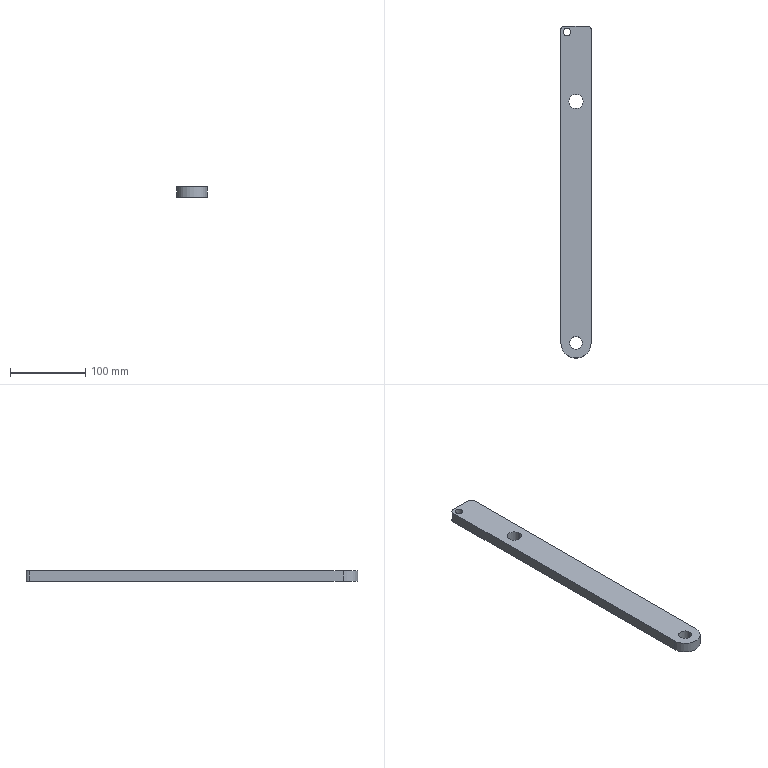Part | SolidWorks | features Extrusion 1, ICE 1 | 1 solid | 14 faces | box 40 x 440 x 14 mm | volume 235600 mm3 | cylinder 9 | plane 5 | commonest cylinder face diameters 10 x4 17 x2 19 x2 40 x1
STEP:
#1=CARTESIAN_POINT('',(-7.,212.,14.));
#2=VERTEX_POINT('',#1);
#3=CARTESIAN_POINT('',(-17.,212.,14.));
#4=VERTEX_POINT('',#3);
#5=CARTESIAN_POINT('',(-12.,212.,14.));
#6=DIRECTION('',(0.,0.,-1.));
#7=DIRECTION('',(-1.,0.,0.));
#8=AXIS2_PLACEMENT_3D('',#5,#6,#7);
#9=CIRCLE('',#8,5.);
#10=EDGE_CURVE('',#2,#4,#9,.T.);
#11=ORIENTED_EDGE('',*,*,#10,.F.);
#12=CARTESIAN_POINT('',(-7.,212.,0.));
#13=VERTEX_POINT('',#12);
#14=CARTESIAN_POINT('',(-7.,212.,20.));
#15=DIRECTION('',(0.,0.,-1.));
#16=VECTOR('',#15,1000.);
#17=LINE('',#14,#16);
#18=EDGE_CURVE('',#2,#13,#17,.T.);
#19=ORIENTED_EDGE('',*,*,#18,.T.);
#20=CARTESIAN_POINT('',(-17.,212.,0.));
#21=VERTEX_POINT('',#20);
#22=CARTESIAN_POINT('',(-12.,212.,0.));
#23=DIRECTION('',(0.,0.,-1.));
#24=DIRECTION('',(-1.,0.,0.));
#25=AXIS2_PLACEMENT_3D('',#22,#23,#24);
#26=CIRCLE('',#25,5.);
#27=EDGE_CURVE('',#13,#21,#26,.T.);
#28=ORIENTED_EDGE('',*,*,#27,.T.);
#29=CARTESIAN_POINT('',(-17.,212.,20.));
#30=DIRECTION('',(0.,0.,-1.));
#31=VECTOR('',#30,1000.);
#32=LINE('',#29,#31);
#33=EDGE_CURVE('',#4,#21,#32,.T.);
#34=ORIENTED_EDGE('',*,*,#33,.F.);
#35=EDGE_LOOP('',(#11,#19,#28,#34));
#36=FACE_OUTER_BOUND('',#35,.T.);
#37=CARTESIAN_POINT('',(-12.,212.,20.));
#38=DIRECTION('',(0.,0.,-1.));
#39=DIRECTION('',(-1.,0.,0.));
#40=AXIS2_PLACEMENT_3D('',#37,#38,#39);
#41=CYLINDRICAL_SURFACE('',#40,5.);
#42=ADVANCED_FACE('',(#36),#41,.F.);
#43=CARTESIAN_POINT('',(-8.5,-200.,14.));
#44=VERTEX_POINT('',#43);
#45=CARTESIAN_POINT('',(8.5,-200.,14.));
#46=VERTEX_POINT('',#45);
#47=CARTESIAN_POINT('',(0.,-200.,14.));
#48=DIRECTION('',(0.,0.,1.));
#49=DIRECTION('',(1.,0.,0.));
#50=AXIS2_PLACEMENT_3D('',#47,#48,#49);
#51=CIRCLE('',#50,8.5);
#52=EDGE_CURVE('',#44,#46,#51,.T.);
#53=ORIENTED_EDGE('',*,*,#52,.T.);
#54=CARTESIAN_POINT('',(8.5,-200.,0.));
#55=VERTEX_POINT('',#54);
#56=CARTESIAN_POINT('',(8.5,-200.,14.));
#57=DIRECTION('',(0.,0.,-1.));
#58=VECTOR('',#57,1000.);
#59=LINE('',#56,#58);
#60=EDGE_CURVE('',#46,#55,#59,.T.);
#61=ORIENTED_EDGE('',*,*,#60,.T.);
#62=CARTESIAN_POINT('',(-8.5,-200.,0.));
#63=VERTEX_POINT('',#62);
#64=CARTESIAN_POINT('',(0.,-200.,0.));
#65=DIRECTION('',(0.,0.,1.));
#66=DIRECTION('',(1.,0.,0.));
#67=AXIS2_PLACEMENT_3D('',#64,#65,#66);
#68=CIRCLE('',#67,8.5);
#69=EDGE_CURVE('',#63,#55,#68,.T.);
#70=ORIENTED_EDGE('',*,*,#69,.F.);
#71=CARTESIAN_POINT('',(-8.5,-200.,14.));
#72=DIRECTION('',(0.,0.,-1.));
#73=VECTOR('',#72,1000.);
#74=LINE('',#71,#73);
#75=EDGE_CURVE('',#44,#63,#74,.T.);
#76=ORIENTED_EDGE('',*,*,#75,.F.);
#77=EDGE_LOOP('',(#53,#61,#70,#76));
#78=FACE_OUTER_BOUND('',#77,.T.);
#79=CARTESIAN_POINT('',(0.,-200.,14.));
#80=DIRECTION('',(0.,0.,-1.));
#81=DIRECTION('',(-1.,0.,0.));
#82=AXIS2_PLACEMENT_3D('',#79,#80,#81);
#83=CYLINDRICAL_SURFACE('',#82,8.5);
#84=ADVANCED_FACE('',(#78),#83,.F.);
#85=CARTESIAN_POINT('',(-9.5,120.,14.));
#86=VERTEX_POINT('',#85);
#87=CARTESIAN_POINT('',(9.5,120.,14.));
#88=VERTEX_POINT('',#87);
#89=CARTESIAN_POINT('',(0.,120.,14.));
#90=DIRECTION('',(0.,0.,1.));
#91=DIRECTION('',(1.,0.,0.));
#92=AXIS2_PLACEMENT_3D('',#89,#90,#91);
#93=CIRCLE('',#92,9.5);
#94=EDGE_CURVE('',#86,#88,#93,.T.);
#95=ORIENTED_EDGE('',*,*,#94,.T.);
#96=CARTESIAN_POINT('',(9.5,120.,0.));
#97=VERTEX_POINT('',#96);
#98=CARTESIAN_POINT('',(9.5,120.,14.));
#99=DIRECTION('',(0.,0.,-1.));
#100=VECTOR('',#99,1000.);
#101=LINE('',#98,#100);
#102=EDGE_CURVE('',#88,#97,#101,.T.);
#103=ORIENTED_EDGE('',*,*,#102,.T.);
#104=CARTESIAN_POINT('',(-9.5,120.,0.));
#105=VERTEX_POINT('',#104);
#106=CARTESIAN_POINT('',(0.,120.,0.));
#107=DIRECTION('',(0.,0.,1.));
#108=DIRECTION('',(1.,0.,0.));
#109=AXIS2_PLACEMENT_3D('',#106,#107,#108);
#110=CIRCLE('',#109,9.5);
#111=EDGE_CURVE('',#105,#97,#110,.T.);
#112=ORIENTED_EDGE('',*,*,#111,.F.);
#113=CARTESIAN_POINT('',(-9.5,120.,14.));
#114=DIRECTION('',(0.,0.,-1.));
#115=VECTOR('',#114,1000.);
#116=LINE('',#113,#115);
#117=EDGE_CURVE('',#86,#105,#116,.T.);
#118=ORIENTED_EDGE('',*,*,#117,.F.);
#119=EDGE_LOOP('',(#95,#103,#112,#118));
#120=FACE_OUTER_BOUND('',#119,.T.);
#121=CARTESIAN_POINT('',(0.,120.,14.));
#122=DIRECTION('',(0.,0.,-1.));
#123=DIRECTION('',(-1.,0.,0.));
#124=AXIS2_PLACEMENT_3D('',#121,#122,#123);
#125=CYLINDRICAL_SURFACE('',#124,9.5);
#126=ADVANCED_FACE('',(#120),#125,.F.);
#127=CARTESIAN_POINT('',(-12.,212.,14.));
#128=DIRECTION('',(0.,0.,-1.));
#129=DIRECTION('',(-1.,0.,0.));
#130=AXIS2_PLACEMENT_3D('',#127,#128,#129);
#131=CIRCLE('',#130,5.);
#132=EDGE_CURVE('',#4,#2,#131,.T.);
#133=ORIENTED_EDGE('',*,*,#132,.T.);
#134=ORIENTED_EDGE('',*,*,#10,.T.);
#135=EDGE_LOOP('',(#133,#134));
#136=FACE_BOUND('',#135,.T.);
#137=CARTESIAN_POINT('',(20.,215.,14.));
#138=VERTEX_POINT('',#137);
#139=CARTESIAN_POINT('',(15.,220.,14.));
#140=VERTEX_POINT('',#139);
#141=CARTESIAN_POINT('',(15.,215.,14.));
#142=DIRECTION('',(0.,0.,1.));
#143=DIRECTION('',(-1.,0.,0.));
#144=AXIS2_PLACEMENT_3D('',#141,#142,#143);
#145=CIRCLE('',#144,5.);
#146=EDGE_CURVE('',#138,#140,#145,.T.);
#147=ORIENTED_EDGE('',*,*,#146,.T.);
#148=CARTESIAN_POINT('',(-15.,220.,14.));
#149=VERTEX_POINT('',#148);
#150=CARTESIAN_POINT('',(-15.,220.,14.));
#151=DIRECTION('',(-1.,0.,0.));
#152=VECTOR('',#151,1000.);
#153=LINE('',#150,#152);
#154=EDGE_CURVE('',#140,#149,#153,.T.);
#155=ORIENTED_EDGE('',*,*,#154,.T.);
#156=CARTESIAN_POINT('',(-20.,215.,14.));
#157=VERTEX_POINT('',#156);
#158=CARTESIAN_POINT('',(-15.,215.,14.));
#159=DIRECTION('',(0.,0.,1.));
#160=DIRECTION('',(1.,0.,0.));
#161=AXIS2_PLACEMENT_3D('',#158,#159,#160);
#162=CIRCLE('',#161,5.);
#163=EDGE_CURVE('',#149,#157,#162,.T.);
#164=ORIENTED_EDGE('',*,*,#163,.T.);
#165=CARTESIAN_POINT('',(-20.,-200.,14.));
#166=VERTEX_POINT('',#165);
#167=CARTESIAN_POINT('',(-20.,215.,14.));
#168=DIRECTION('',(0.,-1.,0.));
#169=VECTOR('',#168,1000.);
#170=LINE('',#167,#169);
#171=EDGE_CURVE('',#157,#166,#170,.T.);
#172=ORIENTED_EDGE('',*,*,#171,.T.);
#173=CARTESIAN_POINT('',(20.,-200.,14.));
#174=VERTEX_POINT('',#173);
#175=CARTESIAN_POINT('',(0.,-200.,14.));
#176=DIRECTION('',(0.,0.,1.));
#177=DIRECTION('',(1.,0.,0.));
#178=AXIS2_PLACEMENT_3D('',#175,#176,#177);
#179=CIRCLE('',#178,20.);
#180=EDGE_CURVE('',#166,#174,#179,.T.);
#181=ORIENTED_EDGE('',*,*,#180,.T.);
#182=CARTESIAN_POINT('',(20.,215.,14.));
#183=DIRECTION('',(0.,1.,0.));
#184=VECTOR('',#183,1000.);
#185=LINE('',#182,#184);
#186=EDGE_CURVE('',#174,#138,#185,.T.);
#187=ORIENTED_EDGE('',*,*,#186,.T.);
#188=EDGE_LOOP('',(#147,#155,#164,#172,#181,#187));
#189=FACE_OUTER_BOUND('',#188,.T.);
#190=ORIENTED_EDGE('',*,*,#94,.F.);
#191=CARTESIAN_POINT('',(0.,120.,14.));
#192=DIRECTION('',(0.,0.,1.));
#193=DIRECTION('',(1.,0.,0.));
#194=AXIS2_PLACEMENT_3D('',#191,#192,#193);
#195=CIRCLE('',#194,9.5);
#196=EDGE_CURVE('',#88,#86,#195,.T.);
#197=ORIENTED_EDGE('',*,*,#196,.F.);
#198=EDGE_LOOP('',(#190,#197));
#199=FACE_BOUND('',#198,.T.);
#200=ORIENTED_EDGE('',*,*,#52,.F.);
#201=CARTESIAN_POINT('',(0.,-200.,14.));
#202=DIRECTION('',(0.,0.,1.));
#203=DIRECTION('',(1.,0.,0.));
#204=AXIS2_PLACEMENT_3D('',#201,#202,#203);
#205=CIRCLE('',#204,8.5);
#206=EDGE_CURVE('',#46,#44,#205,.T.);
#207=ORIENTED_EDGE('',*,*,#206,.F.);
#208=EDGE_LOOP('',(#200,#207));
#209=FACE_BOUND('',#208,.T.);
#210=CARTESIAN_POINT('',(15.,215.,14.));
#211=DIRECTION('',(0.,0.,-1.));
#212=DIRECTION('',(-1.,0.,0.));
#213=AXIS2_PLACEMENT_3D('',#210,#211,#212);
#214=PLANE('',#213);
#215=ADVANCED_FACE('',(#136,#189,#199,#209),#214,.F.);
#216=CARTESIAN_POINT('',(-12.,212.,0.));
#217=DIRECTION('',(0.,0.,-1.));
#218=DIRECTION('',(-1.,0.,0.));
#219=AXIS2_PLACEMENT_3D('',#216,#217,#218);
#220=CIRCLE('',#219,5.);
#221=EDGE_CURVE('',#21,#13,#220,.T.);
#222=ORIENTED_EDGE('',*,*,#221,.F.);
#223=ORIENTED_EDGE('',*,*,#27,.F.);
#224=EDGE_LOOP('',(#222,#223));
#225=FACE_BOUND('',#224,.T.);
#226=ORIENTED_EDGE('',*,*,#111,.T.);
#227=CARTESIAN_POINT('',(0.,120.,0.));
#228=DIRECTION('',(0.,0.,1.));
#229=DIRECTION('',(1.,0.,0.));
#230=AXIS2_PLACEMENT_3D('',#227,#228,#229);
#231=CIRCLE('',#230,9.5);
#232=EDGE_CURVE('',#97,#105,#231,.T.);
#233=ORIENTED_EDGE('',*,*,#232,.T.);
#234=EDGE_LOOP('',(#226,#233));
#235=FACE_BOUND('',#234,.T.);
#236=CARTESIAN_POINT('',(20.,215.,0.));
#237=VERTEX_POINT('',#236);
#238=CARTESIAN_POINT('',(15.,220.,0.));
#239=VERTEX_POINT('',#238);
#240=CARTESIAN_POINT('',(15.,215.,0.));
#241=DIRECTION('',(0.,0.,1.));
#242=DIRECTION('',(-1.,0.,0.));
#243=AXIS2_PLACEMENT_3D('',#240,#241,#242);
#244=CIRCLE('',#243,5.);
#245=EDGE_CURVE('',#237,#239,#244,.T.);
#246=ORIENTED_EDGE('',*,*,#245,.F.);
#247=CARTESIAN_POINT('',(20.,-200.,0.));
#248=VERTEX_POINT('',#247);
#249=CARTESIAN_POINT('',(20.,215.,0.));
#250=DIRECTION('',(0.,1.,0.));
#251=VECTOR('',#250,1000.);
#252=LINE('',#249,#251);
#253=EDGE_CURVE('',#248,#237,#252,.T.);
#254=ORIENTED_EDGE('',*,*,#253,.F.);
#255=CARTESIAN_POINT('',(-20.,-200.,0.));
#256=VERTEX_POINT('',#255);
#257=CARTESIAN_POINT('',(0.,-200.,0.));
#258=DIRECTION('',(0.,0.,1.));
#259=DIRECTION('',(1.,0.,0.));
#260=AXIS2_PLACEMENT_3D('',#257,#258,#259);
#261=CIRCLE('',#260,20.);
#262=EDGE_CURVE('',#256,#248,#261,.T.);
#263=ORIENTED_EDGE('',*,*,#262,.F.);
#264=CARTESIAN_POINT('',(-20.,215.,0.));
#265=VERTEX_POINT('',#264);
#266=CARTESIAN_POINT('',(-20.,215.,0.));
#267=DIRECTION('',(0.,-1.,0.));
#268=VECTOR('',#267,1000.);
#269=LINE('',#266,#268);
#270=EDGE_CURVE('',#265,#256,#269,.T.);
#271=ORIENTED_EDGE('',*,*,#270,.F.);
#272=CARTESIAN_POINT('',(-15.,220.,0.));
#273=VERTEX_POINT('',#272);
#274=CARTESIAN_POINT('',(-15.,215.,0.));
#275=DIRECTION('',(0.,0.,1.));
#276=DIRECTION('',(1.,0.,0.));
#277=AXIS2_PLACEMENT_3D('',#274,#275,#276);
#278=CIRCLE('',#277,5.);
#279=EDGE_CURVE('',#273,#265,#278,.T.);
#280=ORIENTED_EDGE('',*,*,#279,.F.);
#281=CARTESIAN_POINT('',(-15.,220.,0.));
#282=DIRECTION('',(-1.,0.,0.));
#283=VECTOR('',#282,1000.);
#284=LINE('',#281,#283);
#285=EDGE_CURVE('',#239,#273,#284,.T.);
#286=ORIENTED_EDGE('',*,*,#285,.F.);
#287=EDGE_LOOP('',(#246,#254,#263,#271,#280,#286));
#288=FACE_OUTER_BOUND('',#287,.T.);
#289=ORIENTED_EDGE('',*,*,#69,.T.);
#290=CARTESIAN_POINT('',(0.,-200.,0.));
#291=DIRECTION('',(0.,0.,1.));
#292=DIRECTION('',(1.,0.,0.));
#293=AXIS2_PLACEMENT_3D('',#290,#291,#292);
#294=CIRCLE('',#293,8.5);
#295=EDGE_CURVE('',#55,#63,#294,.T.);
#296=ORIENTED_EDGE('',*,*,#295,.T.);
#297=EDGE_LOOP('',(#289,#296));
#298=FACE_BOUND('',#297,.T.);
#299=CARTESIAN_POINT('',(15.,215.,0.));
#300=DIRECTION('',(0.,0.,-1.));
#301=DIRECTION('',(-1.,0.,0.));
#302=AXIS2_PLACEMENT_3D('',#299,#300,#301);
#303=PLANE('',#302);
#304=ADVANCED_FACE('',(#225,#235,#288,#298),#303,.T.);
#305=ORIENTED_EDGE('',*,*,#245,.T.);
#306=CARTESIAN_POINT('',(15.,220.,14.));
#307=DIRECTION('',(0.,0.,-1.));
#308=VECTOR('',#307,1000.);
#309=LINE('',#306,#308);
#310=EDGE_CURVE('',#140,#239,#309,.T.);
#311=ORIENTED_EDGE('',*,*,#310,.F.);
#312=ORIENTED_EDGE('',*,*,#146,.F.);
#313=CARTESIAN_POINT('',(20.,215.,14.));
#314=DIRECTION('',(0.,0.,-1.));
#315=VECTOR('',#314,1000.);
#316=LINE('',#313,#315);
#317=EDGE_CURVE('',#138,#237,#316,.T.);
#318=ORIENTED_EDGE('',*,*,#317,.T.);
#319=EDGE_LOOP('',(#305,#311,#312,#318));
#320=FACE_OUTER_BOUND('',#319,.T.);
#321=CARTESIAN_POINT('',(15.,215.,14.));
#322=DIRECTION('',(0.,0.,-1.));
#323=DIRECTION('',(-1.,0.,0.));
#324=AXIS2_PLACEMENT_3D('',#321,#322,#323);
#325=CYLINDRICAL_SURFACE('',#324,5.);
#326=ADVANCED_FACE('',(#320),#325,.T.);
#327=ORIENTED_EDGE('',*,*,#285,.T.);
#328=CARTESIAN_POINT('',(-15.,220.,14.));
#329=DIRECTION('',(0.,0.,-1.));
#330=VECTOR('',#329,1000.);
#331=LINE('',#328,#330);
#332=EDGE_CURVE('',#149,#273,#331,.T.);
#333=ORIENTED_EDGE('',*,*,#332,.F.);
#334=ORIENTED_EDGE('',*,*,#154,.F.);
#335=ORIENTED_EDGE('',*,*,#310,.T.);
#336=EDGE_LOOP('',(#327,#333,#334,#335));
#337=FACE_OUTER_BOUND('',#336,.T.);
#338=CARTESIAN_POINT('',(-15.,220.,14.));
#339=DIRECTION('',(0.,-1.,0.));
#340=DIRECTION('',(0.,0.,-1.));
#341=AXIS2_PLACEMENT_3D('',#338,#339,#340);
#342=PLANE('',#341);
#343=ADVANCED_FACE('',(#337),#342,.F.);
#344=ORIENTED_EDGE('',*,*,#279,.T.);
#345=CARTESIAN_POINT('',(-20.,215.,14.));
#346=DIRECTION('',(0.,0.,-1.));
#347=VECTOR('',#346,1000.);
#348=LINE('',#345,#347);
#349=EDGE_CURVE('',#157,#265,#348,.T.);
#350=ORIENTED_EDGE('',*,*,#349,.F.);
#351=ORIENTED_EDGE('',*,*,#163,.F.);
#352=ORIENTED_EDGE('',*,*,#332,.T.);
#353=EDGE_LOOP('',(#344,#350,#351,#352));
#354=FACE_OUTER_BOUND('',#353,.T.);
#355=CARTESIAN_POINT('',(-15.,215.,14.));
#356=DIRECTION('',(0.,0.,-1.));
#357=DIRECTION('',(-1.,0.,0.));
#358=AXIS2_PLACEMENT_3D('',#355,#356,#357);
#359=CYLINDRICAL_SURFACE('',#358,5.);
#360=ADVANCED_FACE('',(#354),#359,.T.);
#361=ORIENTED_EDGE('',*,*,#270,.T.);
#362=CARTESIAN_POINT('',(-20.,-200.,14.));
#363=DIRECTION('',(0.,0.,-1.));
#364=VECTOR('',#363,1000.);
#365=LINE('',#362,#364);
#366=EDGE_CURVE('',#166,#256,#365,.T.);
#367=ORIENTED_EDGE('',*,*,#366,.F.);
#368=ORIENTED_EDGE('',*,*,#171,.F.);
#369=ORIENTED_EDGE('',*,*,#349,.T.);
#370=EDGE_LOOP('',(#361,#367,#368,#369));
#371=FACE_OUTER_BOUND('',#370,.T.);
#372=CARTESIAN_POINT('',(-20.,215.,14.));
#373=DIRECTION('',(1.,0.,0.));
#374=DIRECTION('',(0.,1.,0.));
#375=AXIS2_PLACEMENT_3D('',#372,#373,#374);
#376=PLANE('',#375);
#377=ADVANCED_FACE('',(#371),#376,.F.);
#378=ORIENTED_EDGE('',*,*,#262,.T.);
#379=CARTESIAN_POINT('',(20.,-200.,14.));
#380=DIRECTION('',(0.,0.,-1.));
#381=VECTOR('',#380,1000.);
#382=LINE('',#379,#381);
#383=EDGE_CURVE('',#174,#248,#382,.T.);
#384=ORIENTED_EDGE('',*,*,#383,.F.);
#385=ORIENTED_EDGE('',*,*,#180,.F.);
#386=ORIENTED_EDGE('',*,*,#366,.T.);
#387=EDGE_LOOP('',(#378,#384,#385,#386));
#388=FACE_OUTER_BOUND('',#387,.T.);
#389=CARTESIAN_POINT('',(0.,-200.,14.));
#390=DIRECTION('',(0.,0.,-1.));
#391=DIRECTION('',(-1.,0.,0.));
#392=AXIS2_PLACEMENT_3D('',#389,#390,#391);
#393=CYLINDRICAL_SURFACE('',#392,20.);
#394=ADVANCED_FACE('',(#388),#393,.T.);
#395=ORIENTED_EDGE('',*,*,#253,.T.);
#396=ORIENTED_EDGE('',*,*,#317,.F.);
#397=ORIENTED_EDGE('',*,*,#186,.F.);
#398=ORIENTED_EDGE('',*,*,#383,.T.);
#399=EDGE_LOOP('',(#395,#396,#397,#398));
#400=FACE_OUTER_BOUND('',#399,.T.);
#401=CARTESIAN_POINT('',(20.,215.,14.));
#402=DIRECTION('',(-1.,0.,0.));
#403=DIRECTION('',(0.,-1.,0.));
#404=AXIS2_PLACEMENT_3D('',#401,#402,#403);
#405=PLANE('',#404);
#406=ADVANCED_FACE('',(#400),#405,.F.);
#407=ORIENTED_EDGE('',*,*,#102,.F.);
#408=ORIENTED_EDGE('',*,*,#196,.T.);
#409=ORIENTED_EDGE('',*,*,#117,.T.);
#410=ORIENTED_EDGE('',*,*,#232,.F.);
#411=EDGE_LOOP('',(#407,#408,#409,#410));
#412=FACE_OUTER_BOUND('',#411,.T.);
#413=CARTESIAN_POINT('',(0.,120.,14.));
#414=DIRECTION('',(0.,0.,-1.));
#415=DIRECTION('',(-1.,0.,0.));
#416=AXIS2_PLACEMENT_3D('',#413,#414,#415);
#417=CYLINDRICAL_SURFACE('',#416,9.5);
#418=ADVANCED_FACE('',(#412),#417,.F.);
#419=ORIENTED_EDGE('',*,*,#60,.F.);
#420=ORIENTED_EDGE('',*,*,#206,.T.);
#421=ORIENTED_EDGE('',*,*,#75,.T.);
#422=ORIENTED_EDGE('',*,*,#295,.F.);
#423=EDGE_LOOP('',(#419,#420,#421,#422));
#424=FACE_OUTER_BOUND('',#423,.T.);
#425=CARTESIAN_POINT('',(0.,-200.,14.));
#426=DIRECTION('',(0.,0.,-1.));
#427=DIRECTION('',(-1.,0.,0.));
#428=AXIS2_PLACEMENT_3D('',#425,#426,#427);
#429=CYLINDRICAL_SURFACE('',#428,8.5);
#430=ADVANCED_FACE('',(#424),#429,.F.);
#431=ORIENTED_EDGE('',*,*,#18,.F.);
#432=ORIENTED_EDGE('',*,*,#132,.F.);
#433=ORIENTED_EDGE('',*,*,#33,.T.);
#434=ORIENTED_EDGE('',*,*,#221,.T.);
#435=EDGE_LOOP('',(#431,#432,#433,#434));
#436=FACE_OUTER_BOUND('',#435,.T.);
#437=CARTESIAN_POINT('',(-12.,212.,20.));
#438=DIRECTION('',(0.,0.,-1.));
#439=DIRECTION('',(-1.,0.,0.));
#440=AXIS2_PLACEMENT_3D('',#437,#438,#439);
#441=CYLINDRICAL_SURFACE('',#440,5.);
#442=ADVANCED_FACE('',(#436),#441,.F.);
#443=CLOSED_SHELL('',(#42,#84,#126,#215,#304,#326,#343,#360,#377,#394,#406,#418,#430,#442));
#444=MANIFOLD_SOLID_BREP('',#443);
#445=CARTESIAN_POINT('',(0.,0.,0.));
#446=DIRECTION('',(0.,0.,1.));
#447=DIRECTION('',(1.,0.,0.));
#448=AXIS2_PLACEMENT_3D('',#445,#446,#447);
#449=(LENGTH_UNIT()NAMED_UNIT(*)SI_UNIT(.MILLI.,.METRE.));
#450=UNCERTAINTY_MEASURE_WITH_UNIT(LENGTH_MEASURE(0.00001),#449,'','');
#451=(NAMED_UNIT(*)PLANE_ANGLE_UNIT()SI_UNIT($,.RADIAN.));
#452=(NAMED_UNIT(*)SI_UNIT($,.STERADIAN.)SOLID_ANGLE_UNIT());
#453=(GEOMETRIC_REPRESENTATION_CONTEXT(3)GLOBAL_UNCERTAINTY_ASSIGNED_CONTEXT((#450))GLOBAL_UNIT_ASSIGNED_CONTEXT((#449,#451,#452))REPRESENTATION_CONTEXT('',''));
#454=ADVANCED_BREP_SHAPE_REPRESENTATION('',(#444,#448),#453);